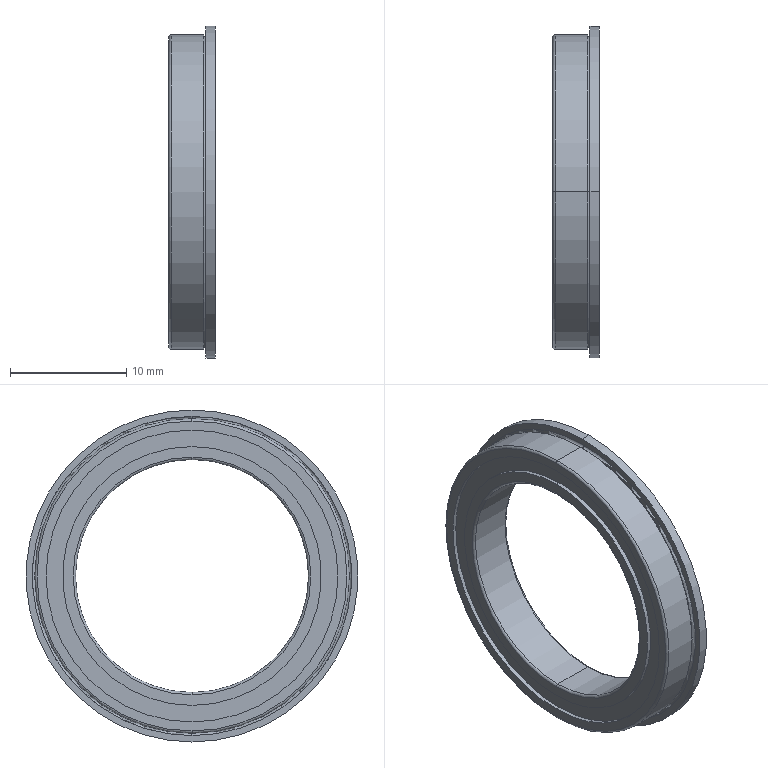Part | NX | features BREP 1 | 1 solid | 31 faces | box 4 x 28.5 x 28.5 mm | volume 1002 mm3 | cylinder 14 | torus 10 | plane 7 | commonest cylinder face diameters 22.21 x4 25.05 x4 20 x2 27 x2 28.5 x2
STEP:
#1=CARTESIAN_POINT('',(0.,0.,13.3));
#2=VERTEX_POINT('',#1);
#3=CARTESIAN_POINT('',(-0.2,0.,13.5));
#4=VERTEX_POINT('',#3);
#5=CARTESIAN_POINT('',(0.,0.,13.5));
#6=DIRECTION('',(0.,-1.,0.));
#7=DIRECTION('',(0.,0.,-1.));
#8=AXIS2_PLACEMENT_3D('',#5,#6,#7);
#9=CIRCLE('',#8,0.2);
#10=EDGE_CURVE('',#2,#4,#9,.F.);
#11=ORIENTED_EDGE('',*,*,#10,.F.);
#12=CARTESIAN_POINT('',(0.,0.,-13.3));
#13=VERTEX_POINT('',#12);
#14=CARTESIAN_POINT('',(0.,0.,0.));
#15=DIRECTION('',(-1.,0.,0.));
#16=DIRECTION('',(0.,0.,1.));
#17=AXIS2_PLACEMENT_3D('',#14,#15,#16);
#18=CIRCLE('',#17,13.3);
#19=EDGE_CURVE('',#2,#13,#18,.T.);
#20=ORIENTED_EDGE('',*,*,#19,.T.);
#21=CARTESIAN_POINT('',(-0.2,0.,-13.5));
#22=VERTEX_POINT('',#21);
#23=CARTESIAN_POINT('',(0.,0.,-13.5));
#24=DIRECTION('',(0.,1.,0.));
#25=DIRECTION('',(0.,0.,1.));
#26=AXIS2_PLACEMENT_3D('',#23,#24,#25);
#27=CIRCLE('',#26,0.2);
#28=EDGE_CURVE('',#13,#22,#27,.F.);
#29=ORIENTED_EDGE('',*,*,#28,.T.);
#30=CARTESIAN_POINT('',(-0.2,0.,0.));
#31=DIRECTION('',(-1.,0.,0.));
#32=DIRECTION('',(0.,0.,1.));
#33=AXIS2_PLACEMENT_3D('',#30,#31,#32);
#34=CIRCLE('',#33,13.5);
#35=EDGE_CURVE('',#4,#22,#34,.T.);
#36=ORIENTED_EDGE('',*,*,#35,.F.);
#37=EDGE_LOOP('',(#11,#20,#29,#36));
#38=FACE_BOUND('',#37,.T.);
#39=CARTESIAN_POINT('',(0.,0.,0.));
#40=DIRECTION('',(-1.,0.,0.));
#41=DIRECTION('',(0.,0.,-1.));
#42=AXIS2_PLACEMENT_3D('',#39,#40,#41);
#43=TOROIDAL_SURFACE('',#42,13.5,0.2);
#44=ADVANCED_FACE('',(#38),#43,.F.);
#45=ORIENTED_EDGE('',*,*,#28,.F.);
#46=CARTESIAN_POINT('',(0.,0.,0.));
#47=DIRECTION('',(-1.,0.,0.));
#48=DIRECTION('',(0.,0.,1.));
#49=AXIS2_PLACEMENT_3D('',#46,#47,#48);
#50=CIRCLE('',#49,13.3);
#51=EDGE_CURVE('',#13,#2,#50,.T.);
#52=ORIENTED_EDGE('',*,*,#51,.T.);
#53=ORIENTED_EDGE('',*,*,#10,.T.);
#54=CARTESIAN_POINT('',(-0.2,0.,0.));
#55=DIRECTION('',(-1.,0.,0.));
#56=DIRECTION('',(0.,0.,1.));
#57=AXIS2_PLACEMENT_3D('',#54,#55,#56);
#58=CIRCLE('',#57,13.5);
#59=EDGE_CURVE('',#22,#4,#58,.T.);
#60=ORIENTED_EDGE('',*,*,#59,.F.);
#61=EDGE_LOOP('',(#45,#52,#53,#60));
#62=FACE_BOUND('',#61,.T.);
#63=CARTESIAN_POINT('',(0.,0.,0.));
#64=DIRECTION('',(-1.,0.,0.));
#65=DIRECTION('',(0.,0.,-1.));
#66=AXIS2_PLACEMENT_3D('',#63,#64,#65);
#67=TOROIDAL_SURFACE('',#66,13.5,0.2);
#68=ADVANCED_FACE('',(#62),#67,.F.);
#69=CARTESIAN_POINT('',(-3.2,0.,13.3));
#70=VERTEX_POINT('',#69);
#71=CARTESIAN_POINT('',(-3.2,0.,-13.3));
#72=VERTEX_POINT('',#71);
#73=CARTESIAN_POINT('',(-3.2,0.,0.));
#74=DIRECTION('',(-1.,0.,0.));
#75=DIRECTION('',(0.,0.,-1.));
#76=AXIS2_PLACEMENT_3D('',#73,#74,#75);
#77=CIRCLE('',#76,13.3);
#78=EDGE_CURVE('',#70,#72,#77,.T.);
#79=ORIENTED_EDGE('',*,*,#78,.F.);
#80=CARTESIAN_POINT('',(-3.,0.,13.5));
#81=VERTEX_POINT('',#80);
#82=CARTESIAN_POINT('',(-3.,0.,13.3));
#83=DIRECTION('',(0.,1.,0.));
#84=DIRECTION('',(0.,0.,1.));
#85=AXIS2_PLACEMENT_3D('',#82,#83,#84);
#86=CIRCLE('',#85,0.2);
#87=EDGE_CURVE('',#81,#70,#86,.F.);
#88=ORIENTED_EDGE('',*,*,#87,.F.);
#89=CARTESIAN_POINT('',(-3.,0.,-13.5));
#90=VERTEX_POINT('',#89);
#91=CARTESIAN_POINT('',(-3.,0.,0.));
#92=DIRECTION('',(1.,0.,0.));
#93=DIRECTION('',(0.,0.,-1.));
#94=AXIS2_PLACEMENT_3D('',#91,#92,#93);
#95=CIRCLE('',#94,13.5);
#96=EDGE_CURVE('',#90,#81,#95,.T.);
#97=ORIENTED_EDGE('',*,*,#96,.F.);
#98=CARTESIAN_POINT('',(-3.,0.,-13.3));
#99=DIRECTION('',(0.,-1.,0.));
#100=DIRECTION('',(0.,0.,-1.));
#101=AXIS2_PLACEMENT_3D('',#98,#99,#100);
#102=CIRCLE('',#101,0.2);
#103=EDGE_CURVE('',#90,#72,#102,.F.);
#104=ORIENTED_EDGE('',*,*,#103,.T.);
#105=EDGE_LOOP('',(#79,#88,#97,#104));
#106=FACE_BOUND('',#105,.T.);
#107=CARTESIAN_POINT('',(-3.,0.,0.));
#108=DIRECTION('',(1.,0.,0.));
#109=DIRECTION('',(0.,0.,1.));
#110=AXIS2_PLACEMENT_3D('',#107,#108,#109);
#111=TOROIDAL_SURFACE('',#110,13.3,0.2);
#112=ADVANCED_FACE('',(#106),#111,.T.);
#113=CARTESIAN_POINT('',(-3.,0.,10.));
#114=VERTEX_POINT('',#113);
#115=CARTESIAN_POINT('',(-3.,0.,-10.));
#116=VERTEX_POINT('',#115);
#117=CARTESIAN_POINT('',(-3.,0.,0.));
#118=DIRECTION('',(-1.,0.,0.));
#119=DIRECTION('',(0.,0.,-1.));
#120=AXIS2_PLACEMENT_3D('',#117,#118,#119);
#121=CIRCLE('',#120,10.);
#122=EDGE_CURVE('',#114,#116,#121,.T.);
#123=ORIENTED_EDGE('',*,*,#122,.F.);
#124=CARTESIAN_POINT('',(-3.2,0.,10.2));
#125=VERTEX_POINT('',#124);
#126=CARTESIAN_POINT('',(-3.,0.,10.2));
#127=DIRECTION('',(0.,1.,0.));
#128=DIRECTION('',(0.,0.,1.));
#129=AXIS2_PLACEMENT_3D('',#126,#127,#128);
#130=CIRCLE('',#129,0.2);
#131=EDGE_CURVE('',#125,#114,#130,.F.);
#132=ORIENTED_EDGE('',*,*,#131,.F.);
#133=CARTESIAN_POINT('',(-3.2,0.,-10.2));
#134=VERTEX_POINT('',#133);
#135=CARTESIAN_POINT('',(-3.2,0.,0.));
#136=DIRECTION('',(1.,0.,0.));
#137=DIRECTION('',(0.,0.,-1.));
#138=AXIS2_PLACEMENT_3D('',#135,#136,#137);
#139=CIRCLE('',#138,10.2);
#140=EDGE_CURVE('',#134,#125,#139,.T.);
#141=ORIENTED_EDGE('',*,*,#140,.F.);
#142=CARTESIAN_POINT('',(-3.,0.,-10.2));
#143=DIRECTION('',(0.,-1.,0.));
#144=DIRECTION('',(0.,0.,-1.));
#145=AXIS2_PLACEMENT_3D('',#142,#143,#144);
#146=CIRCLE('',#145,0.2);
#147=EDGE_CURVE('',#134,#116,#146,.F.);
#148=ORIENTED_EDGE('',*,*,#147,.T.);
#149=EDGE_LOOP('',(#123,#132,#141,#148));
#150=FACE_BOUND('',#149,.T.);
#151=CARTESIAN_POINT('',(-3.,0.,0.));
#152=DIRECTION('',(1.,0.,0.));
#153=DIRECTION('',(0.,0.,1.));
#154=AXIS2_PLACEMENT_3D('',#151,#152,#153);
#155=TOROIDAL_SURFACE('',#154,10.2,0.2);
#156=ADVANCED_FACE('',(#150),#155,.T.);
#157=CARTESIAN_POINT('',(0.6,0.,-10.));
#158=VERTEX_POINT('',#157);
#159=CARTESIAN_POINT('',(0.6,0.,10.));
#160=VERTEX_POINT('',#159);
#161=CARTESIAN_POINT('',(0.6,0.,0.));
#162=DIRECTION('',(1.,0.,0.));
#163=DIRECTION('',(0.,0.,1.));
#164=AXIS2_PLACEMENT_3D('',#161,#162,#163);
#165=CIRCLE('',#164,10.);
#166=EDGE_CURVE('',#158,#160,#165,.T.);
#167=ORIENTED_EDGE('',*,*,#166,.F.);
#168=CARTESIAN_POINT('',(0.8,0.,-10.2));
#169=VERTEX_POINT('',#168);
#170=CARTESIAN_POINT('',(0.6,0.,-10.2));
#171=DIRECTION('',(0.,1.,0.));
#172=DIRECTION('',(0.,0.,1.));
#173=AXIS2_PLACEMENT_3D('',#170,#171,#172);
#174=CIRCLE('',#173,0.2);
#175=EDGE_CURVE('',#158,#169,#174,.T.);
#176=ORIENTED_EDGE('',*,*,#175,.T.);
#177=CARTESIAN_POINT('',(0.8,0.,10.2));
#178=VERTEX_POINT('',#177);
#179=CARTESIAN_POINT('',(0.8,0.,0.));
#180=DIRECTION('',(-1.,0.,0.));
#181=DIRECTION('',(0.,0.,1.));
#182=AXIS2_PLACEMENT_3D('',#179,#180,#181);
#183=CIRCLE('',#182,10.2);
#184=EDGE_CURVE('',#178,#169,#183,.T.);
#185=ORIENTED_EDGE('',*,*,#184,.F.);
#186=CARTESIAN_POINT('',(0.6,0.,10.2));
#187=DIRECTION('',(0.,-1.,0.));
#188=DIRECTION('',(0.,0.,-1.));
#189=AXIS2_PLACEMENT_3D('',#186,#187,#188);
#190=CIRCLE('',#189,0.2);
#191=EDGE_CURVE('',#160,#178,#190,.T.);
#192=ORIENTED_EDGE('',*,*,#191,.F.);
#193=EDGE_LOOP('',(#167,#176,#185,#192));
#194=FACE_BOUND('',#193,.T.);
#195=CARTESIAN_POINT('',(0.6,0.,0.));
#196=DIRECTION('',(-1.,0.,0.));
#197=DIRECTION('',(0.,0.,-1.));
#198=AXIS2_PLACEMENT_3D('',#195,#196,#197);
#199=TOROIDAL_SURFACE('',#198,10.2,0.2);
#200=ADVANCED_FACE('',(#194),#199,.T.);
#201=CARTESIAN_POINT('',(0.8,0.,-12.525));
#202=VERTEX_POINT('',#201);
#203=CARTESIAN_POINT('',(0.8,0.,12.525));
#204=VERTEX_POINT('',#203);
#205=CARTESIAN_POINT('',(0.8,0.,0.));
#206=DIRECTION('',(-1.,0.,0.));
#207=DIRECTION('',(0.,0.,1.));
#208=AXIS2_PLACEMENT_3D('',#205,#206,#207);
#209=CIRCLE('',#208,12.525);
#210=EDGE_CURVE('',#202,#204,#209,.T.);
#211=ORIENTED_EDGE('',*,*,#210,.F.);
#212=CARTESIAN_POINT('',(0.45,0.,-12.525));
#213=VERTEX_POINT('',#212);
#214=CARTESIAN_POINT('',(-3.2,0.,-12.525));
#215=DIRECTION('',(-1.,0.,0.));
#216=VECTOR('',#215,1000.);
#217=LINE('',#214,#216);
#218=EDGE_CURVE('',#202,#213,#217,.T.);
#219=ORIENTED_EDGE('',*,*,#218,.T.);
#220=CARTESIAN_POINT('',(0.45,0.,12.525));
#221=VERTEX_POINT('',#220);
#222=CARTESIAN_POINT('',(0.45,0.,0.));
#223=DIRECTION('',(-1.,0.,0.));
#224=DIRECTION('',(0.,0.,1.));
#225=AXIS2_PLACEMENT_3D('',#222,#223,#224);
#226=CIRCLE('',#225,12.525);
#227=EDGE_CURVE('',#213,#221,#226,.T.);
#228=ORIENTED_EDGE('',*,*,#227,.T.);
#229=CARTESIAN_POINT('',(-3.2,0.,12.525));
#230=DIRECTION('',(-1.,0.,0.));
#231=VECTOR('',#230,1000.);
#232=LINE('',#229,#231);
#233=EDGE_CURVE('',#204,#221,#232,.T.);
#234=ORIENTED_EDGE('',*,*,#233,.F.);
#235=EDGE_LOOP('',(#211,#219,#228,#234));
#236=FACE_BOUND('',#235,.T.);
#237=CARTESIAN_POINT('',(-3.2,0.,0.));
#238=DIRECTION('',(-1.,0.,0.));
#239=DIRECTION('',(0.,0.,-1.));
#240=AXIS2_PLACEMENT_3D('',#237,#238,#239);
#241=CYLINDRICAL_SURFACE('',#240,12.525);
#242=ADVANCED_FACE('',(#236),#241,.F.);
#243=CARTESIAN_POINT('',(0.8,0.,11.105));
#244=VERTEX_POINT('',#243);
#245=CARTESIAN_POINT('',(0.8,0.,-11.105));
#246=VERTEX_POINT('',#245);
#247=CARTESIAN_POINT('',(0.8,0.,0.));
#248=DIRECTION('',(-1.,0.,0.));
#249=DIRECTION('',(0.,0.,1.));
#250=AXIS2_PLACEMENT_3D('',#247,#248,#249);
#251=CIRCLE('',#250,11.105);
#252=EDGE_CURVE('',#244,#246,#251,.T.);
#253=ORIENTED_EDGE('',*,*,#252,.T.);
#254=CARTESIAN_POINT('',(0.45,0.,-11.105));
#255=VERTEX_POINT('',#254);
#256=CARTESIAN_POINT('',(-3.2,0.,-11.105));
#257=DIRECTION('',(-1.,0.,0.));
#258=VECTOR('',#257,1000.);
#259=LINE('',#256,#258);
#260=EDGE_CURVE('',#246,#255,#259,.T.);
#261=ORIENTED_EDGE('',*,*,#260,.T.);
#262=CARTESIAN_POINT('',(0.45,0.,11.105));
#263=VERTEX_POINT('',#262);
#264=CARTESIAN_POINT('',(0.45,0.,0.));
#265=DIRECTION('',(-1.,0.,0.));
#266=DIRECTION('',(0.,0.,1.));
#267=AXIS2_PLACEMENT_3D('',#264,#265,#266);
#268=CIRCLE('',#267,11.105);
#269=EDGE_CURVE('',#263,#255,#268,.T.);
#270=ORIENTED_EDGE('',*,*,#269,.F.);
#271=CARTESIAN_POINT('',(-3.2,0.,11.105));
#272=DIRECTION('',(-1.,0.,0.));
#273=VECTOR('',#272,1000.);
#274=LINE('',#271,#273);
#275=EDGE_CURVE('',#244,#263,#274,.T.);
#276=ORIENTED_EDGE('',*,*,#275,.F.);
#277=EDGE_LOOP('',(#253,#261,#270,#276));
#278=FACE_BOUND('',#277,.T.);
#279=CARTESIAN_POINT('',(-3.2,0.,0.));
#280=DIRECTION('',(-1.,0.,0.));
#281=DIRECTION('',(0.,0.,-1.));
#282=AXIS2_PLACEMENT_3D('',#279,#280,#281);
#283=CYLINDRICAL_SURFACE('',#282,11.105);
#284=ADVANCED_FACE('',(#278),#283,.T.);
#285=CARTESIAN_POINT('',(0.6,0.,0.));
#286=DIRECTION('',(1.,0.,0.));
#287=DIRECTION('',(0.,0.,1.));
#288=AXIS2_PLACEMENT_3D('',#285,#286,#287);
#289=CIRCLE('',#288,10.);
#290=EDGE_CURVE('',#160,#158,#289,.T.);
#291=ORIENTED_EDGE('',*,*,#290,.T.);
#292=CARTESIAN_POINT('',(-3.2,0.,-10.));
#293=DIRECTION('',(-1.,0.,0.));
#294=VECTOR('',#293,1000.);
#295=LINE('',#292,#294);
#296=EDGE_CURVE('',#158,#116,#295,.T.);
#297=ORIENTED_EDGE('',*,*,#296,.T.);
#298=CARTESIAN_POINT('',(-3.,0.,0.));
#299=DIRECTION('',(-1.,0.,0.));
#300=DIRECTION('',(0.,0.,-1.));
#301=AXIS2_PLACEMENT_3D('',#298,#299,#300);
#302=CIRCLE('',#301,10.);
#303=EDGE_CURVE('',#116,#114,#302,.T.);
#304=ORIENTED_EDGE('',*,*,#303,.T.);
#305=CARTESIAN_POINT('',(-3.2,0.,10.));
#306=DIRECTION('',(-1.,0.,0.));
#307=VECTOR('',#306,1000.);
#308=LINE('',#305,#307);
#309=EDGE_CURVE('',#160,#114,#308,.T.);
#310=ORIENTED_EDGE('',*,*,#309,.F.);
#311=EDGE_LOOP('',(#291,#297,#304,#310));
#312=FACE_BOUND('',#311,.T.);
#313=CARTESIAN_POINT('',(-3.2,0.,0.));
#314=DIRECTION('',(-1.,0.,0.));
#315=DIRECTION('',(0.,0.,-1.));
#316=AXIS2_PLACEMENT_3D('',#313,#314,#315);
#317=CYLINDRICAL_SURFACE('',#316,10.);
#318=ADVANCED_FACE('',(#312),#317,.F.);
#319=CARTESIAN_POINT('',(-2.85,0.,11.105));
#320=VERTEX_POINT('',#319);
#321=CARTESIAN_POINT('',(-2.85,0.,-11.105));
#322=VERTEX_POINT('',#321);
#323=CARTESIAN_POINT('',(-2.85,0.,0.));
#324=DIRECTION('',(-1.,0.,0.));
#325=DIRECTION('',(0.,0.,1.));
#326=AXIS2_PLACEMENT_3D('',#323,#324,#325);
#327=CIRCLE('',#326,11.105);
#328=EDGE_CURVE('',#320,#322,#327,.T.);
#329=ORIENTED_EDGE('',*,*,#328,.T.);
#330=CARTESIAN_POINT('',(-3.2,0.,-11.105));
#331=VERTEX_POINT('',#330);
#332=CARTESIAN_POINT('',(-3.2,0.,-11.105));
#333=DIRECTION('',(-1.,0.,0.));
#334=VECTOR('',#333,1000.);
#335=LINE('',#332,#334);
#336=EDGE_CURVE('',#322,#331,#335,.T.);
#337=ORIENTED_EDGE('',*,*,#336,.T.);
#338=CARTESIAN_POINT('',(-3.2,0.,11.105));
#339=VERTEX_POINT('',#338);
#340=CARTESIAN_POINT('',(-3.2,0.,0.));
#341=DIRECTION('',(-1.,0.,0.));
#342=DIRECTION('',(0.,0.,1.));
#343=AXIS2_PLACEMENT_3D('',#340,#341,#342);
#344=CIRCLE('',#343,11.105);
#345=EDGE_CURVE('',#339,#331,#344,.T.);
#346=ORIENTED_EDGE('',*,*,#345,.F.);
#347=CARTESIAN_POINT('',(-3.2,0.,11.105));
#348=DIRECTION('',(-1.,0.,0.));
#349=VECTOR('',#348,1000.);
#350=LINE('',#347,#349);
#351=EDGE_CURVE('',#320,#339,#350,.T.);
#352=ORIENTED_EDGE('',*,*,#351,.F.);
#353=EDGE_LOOP('',(#329,#337,#346,#352));
#354=FACE_BOUND('',#353,.T.);
#355=CARTESIAN_POINT('',(-3.2,0.,0.));
#356=DIRECTION('',(-1.,0.,0.));
#357=DIRECTION('',(0.,0.,-1.));
#358=AXIS2_PLACEMENT_3D('',#355,#356,#357);
#359=CYLINDRICAL_SURFACE('',#358,11.105);
#360=ADVANCED_FACE('',(#354),#359,.T.);
#361=CARTESIAN_POINT('',(-2.85,0.,-12.525));
#362=VERTEX_POINT('',#361);
#363=CARTESIAN_POINT('',(-2.85,0.,12.525));
#364=VERTEX_POINT('',#363);
#365=CARTESIAN_POINT('',(-2.85,0.,0.));
#366=DIRECTION('',(-1.,0.,0.));
#367=DIRECTION('',(0.,0.,1.));
#368=AXIS2_PLACEMENT_3D('',#365,#366,#367);
#369=CIRCLE('',#368,12.525);
#370=EDGE_CURVE('',#362,#364,#369,.T.);
#371=ORIENTED_EDGE('',*,*,#370,.F.);
#372=CARTESIAN_POINT('',(-3.2,0.,-12.525));
#373=VERTEX_POINT('',#372);
#374=CARTESIAN_POINT('',(-3.2,0.,-12.525));
#375=DIRECTION('',(-1.,0.,0.));
#376=VECTOR('',#375,1000.);
#377=LINE('',#374,#376);
#378=EDGE_CURVE('',#362,#373,#377,.T.);
#379=ORIENTED_EDGE('',*,*,#378,.T.);
#380=CARTESIAN_POINT('',(-3.2,0.,12.525));
#381=VERTEX_POINT('',#380);
#382=CARTESIAN_POINT('',(-3.2,0.,0.));
#383=DIRECTION('',(-1.,0.,0.));
#384=DIRECTION('',(0.,0.,1.));
#385=AXIS2_PLACEMENT_3D('',#382,#383,#384);
#386=CIRCLE('',#385,12.525);
#387=EDGE_CURVE('',#373,#381,#386,.T.);
#388=ORIENTED_EDGE('',*,*,#387,.T.);
#389=CARTESIAN_POINT('',(-3.2,0.,12.525));
#390=DIRECTION('',(-1.,0.,0.));
#391=VECTOR('',#390,1000.);
#392=LINE('',#389,#391);
#393=EDGE_CURVE('',#364,#381,#392,.T.);
#394=ORIENTED_EDGE('',*,*,#393,.F.);
#395=EDGE_LOOP('',(#371,#379,#388,#394));
#396=FACE_BOUND('',#395,.T.);
#397=CARTESIAN_POINT('',(-3.2,0.,0.));
#398=DIRECTION('',(-1.,0.,0.));
#399=DIRECTION('',(0.,0.,-1.));
#400=AXIS2_PLACEMENT_3D('',#397,#398,#399);
#401=CYLINDRICAL_SURFACE('',#400,12.525);
#402=ADVANCED_FACE('',(#396),#401,.F.);
#403=ORIENTED_EDGE('',*,*,#35,.T.);
#404=CARTESIAN_POINT('',(-3.2,0.,-13.5));
#405=DIRECTION('',(-1.,0.,0.));
#406=VECTOR('',#405,1000.);
#407=LINE('',#404,#406);
#408=EDGE_CURVE('',#22,#90,#407,.T.);
#409=ORIENTED_EDGE('',*,*,#408,.T.);
#410=ORIENTED_EDGE('',*,*,#96,.T.);
#411=CARTESIAN_POINT('',(-3.2,0.,13.5));
#412=DIRECTION('',(-1.,0.,0.));
#413=VECTOR('',#412,1000.);
#414=LINE('',#411,#413);
#415=EDGE_CURVE('',#4,#81,#414,.T.);
#416=ORIENTED_EDGE('',*,*,#415,.F.);
#417=EDGE_LOOP('',(#403,#409,#410,#416));
#418=FACE_BOUND('',#417,.T.);
#419=CARTESIAN_POINT('',(-3.2,0.,0.));
#420=DIRECTION('',(-1.,0.,0.));
#421=DIRECTION('',(0.,0.,-1.));
#422=AXIS2_PLACEMENT_3D('',#419,#420,#421);
#423=CYLINDRICAL_SURFACE('',#422,13.5);
#424=ADVANCED_FACE('',(#418),#423,.T.);
#425=ORIENTED_EDGE('',*,*,#51,.F.);
#426=CARTESIAN_POINT('',(0.,0.,-13.7));
#427=VERTEX_POINT('',#426);
#428=CARTESIAN_POINT('',(0.,0.,-13.5));
#429=DIRECTION('',(0.,1.,0.));
#430=DIRECTION('',(0.,0.,1.));
#431=AXIS2_PLACEMENT_3D('',#428,#429,#430);
#432=CIRCLE('',#431,0.2);
#433=EDGE_CURVE('',#13,#427,#432,.T.);
#434=ORIENTED_EDGE('',*,*,#433,.T.);
#435=CARTESIAN_POINT('',(0.,0.,13.7));
#436=VERTEX_POINT('',#435);
#437=CARTESIAN_POINT('',(0.,0.,0.));
#438=DIRECTION('',(-1.,0.,0.));
#439=DIRECTION('',(0.,0.,1.));
#440=AXIS2_PLACEMENT_3D('',#437,#438,#439);
#441=CIRCLE('',#440,13.7);
#442=EDGE_CURVE('',#427,#436,#441,.T.);
#443=ORIENTED_EDGE('',*,*,#442,.T.);
#444=CARTESIAN_POINT('',(0.,0.,13.5));
#445=DIRECTION('',(0.,-1.,0.));
#446=DIRECTION('',(0.,0.,-1.));
#447=AXIS2_PLACEMENT_3D('',#444,#445,#446);
#448=CIRCLE('',#447,0.2);
#449=EDGE_CURVE('',#2,#436,#448,.T.);
#450=ORIENTED_EDGE('',*,*,#449,.F.);
#451=EDGE_LOOP('',(#425,#434,#443,#450));
#452=FACE_BOUND('',#451,.T.);
#453=CARTESIAN_POINT('',(0.,0.,0.));
#454=DIRECTION('',(-1.,0.,0.));
#455=DIRECTION('',(0.,0.,-1.));
#456=AXIS2_PLACEMENT_3D('',#453,#454,#455);
#457=TOROIDAL_SURFACE('',#456,13.5,0.2);
#458=ADVANCED_FACE('',(#452),#457,.F.);
#459=CARTESIAN_POINT('',(0.8,0.,14.25));
#460=VERTEX_POINT('',#459);
#461=CARTESIAN_POINT('',(0.8,0.,-14.25));
#462=VERTEX_POINT('',#461);
#463=CARTESIAN_POINT('',(0.8,0.,0.));
#464=DIRECTION('',(-1.,0.,0.));
#465=DIRECTION('',(0.,0.,1.));
#466=AXIS2_PLACEMENT_3D('',#463,#464,#465);
#467=CIRCLE('',#466,14.25);
#468=EDGE_CURVE('',#460,#462,#467,.T.);
#469=ORIENTED_EDGE('',*,*,#468,.T.);
#470=CARTESIAN_POINT('',(0.,0.,-14.25));
#471=VERTEX_POINT('',#470);
#472=CARTESIAN_POINT('',(-3.2,0.,-14.25));
#473=DIRECTION('',(-1.,0.,0.));
#474=VECTOR('',#473,1000.);
#475=LINE('',#472,#474);
#476=EDGE_CURVE('',#462,#471,#475,.T.);
#477=ORIENTED_EDGE('',*,*,#476,.T.);
#478=CARTESIAN_POINT('',(0.,0.,14.25));
#479=VERTEX_POINT('',#478);
#480=CARTESIAN_POINT('',(0.,0.,0.));
#481=DIRECTION('',(-1.,0.,0.));
#482=DIRECTION('',(0.,0.,1.));
#483=AXIS2_PLACEMENT_3D('',#480,#481,#482);
#484=CIRCLE('',#483,14.25);
#485=EDGE_CURVE('',#479,#471,#484,.T.);
#486=ORIENTED_EDGE('',*,*,#485,.F.);
#487=CARTESIAN_POINT('',(-3.2,0.,14.25));
#488=DIRECTION('',(-1.,0.,0.));
#489=VECTOR('',#488,1000.);
#490=LINE('',#487,#489);
#491=EDGE_CURVE('',#460,#479,#490,.T.);
#492=ORIENTED_EDGE('',*,*,#491,.F.);
#493=EDGE_LOOP('',(#469,#477,#486,#492));
#494=FACE_BOUND('',#493,.T.);
#495=CARTESIAN_POINT('',(-3.2,0.,0.));
#496=DIRECTION('',(-1.,0.,0.));
#497=DIRECTION('',(0.,0.,-1.));
#498=AXIS2_PLACEMENT_3D('',#495,#496,#497);
#499=CYLINDRICAL_SURFACE('',#498,14.25);
#500=ADVANCED_FACE('',(#494),#499,.T.);
#501=ORIENTED_EDGE('',*,*,#476,.F.);
#502=CARTESIAN_POINT('',(0.8,0.,0.));
#503=DIRECTION('',(-1.,0.,0.));
#504=DIRECTION('',(0.,0.,1.));
#505=AXIS2_PLACEMENT_3D('',#502,#503,#504);
#506=CIRCLE('',#505,14.25);
#507=EDGE_CURVE('',#462,#460,#506,.T.);
#508=ORIENTED_EDGE('',*,*,#507,.T.);
#509=ORIENTED_EDGE('',*,*,#491,.T.);
#510=CARTESIAN_POINT('',(0.,0.,0.));
#511=DIRECTION('',(-1.,0.,0.));
#512=DIRECTION('',(0.,0.,1.));
#513=AXIS2_PLACEMENT_3D('',#510,#511,#512);
#514=CIRCLE('',#513,14.25);
#515=EDGE_CURVE('',#471,#479,#514,.T.);
#516=ORIENTED_EDGE('',*,*,#515,.F.);
#517=EDGE_LOOP('',(#501,#508,#509,#516));
#518=FACE_BOUND('',#517,.T.);
#519=CARTESIAN_POINT('',(-3.2,0.,0.));
#520=DIRECTION('',(-1.,0.,0.));
#521=DIRECTION('',(0.,0.,-1.));
#522=AXIS2_PLACEMENT_3D('',#519,#520,#521);
#523=CYLINDRICAL_SURFACE('',#522,14.25);
#524=ADVANCED_FACE('',(#518),#523,.T.);
#525=ORIENTED_EDGE('',*,*,#485,.T.);
#526=ORIENTED_EDGE('',*,*,#515,.T.);
#527=EDGE_LOOP('',(#525,#526));
#528=FACE_BOUND('',#527,.T.);
#529=CARTESIAN_POINT('',(0.,0.,0.));
#530=DIRECTION('',(-1.,0.,0.));
#531=DIRECTION('',(0.,0.,1.));
#532=AXIS2_PLACEMENT_3D('',#529,#530,#531);
#533=CIRCLE('',#532,13.7);
#534=EDGE_CURVE('',#436,#427,#533,.T.);
#535=ORIENTED_EDGE('',*,*,#534,.F.);
#536=ORIENTED_EDGE('',*,*,#442,.F.);
#537=EDGE_LOOP('',(#535,#536));
#538=FACE_BOUND('',#537,.T.);
#539=CARTESIAN_POINT('',(0.,13.7,0.));
#540=DIRECTION('',(1.,0.,0.));
#541=DIRECTION('',(0.,-1.,0.));
#542=AXIS2_PLACEMENT_3D('',#539,#540,#541);
#543=PLANE('',#542);
#544=ADVANCED_FACE('',(#528,#538),#543,.F.);
#545=ORIENTED_EDGE('',*,*,#19,.F.);
#546=ORIENTED_EDGE('',*,*,#449,.T.);
#547=ORIENTED_EDGE('',*,*,#534,.T.);
#548=ORIENTED_EDGE('',*,*,#433,.F.);
#549=EDGE_LOOP('',(#545,#546,#547,#548));
#550=FACE_BOUND('',#549,.T.);
#551=CARTESIAN_POINT('',(0.,0.,0.));
#552=DIRECTION('',(-1.,0.,0.));
#553=DIRECTION('',(0.,0.,-1.));
#554=AXIS2_PLACEMENT_3D('',#551,#552,#553);
#555=TOROIDAL_SURFACE('',#554,13.5,0.2);
#556=ADVANCED_FACE('',(#550),#555,.F.);
#557=ORIENTED_EDGE('',*,*,#408,.F.);
#558=ORIENTED_EDGE('',*,*,#59,.T.);
#559=ORIENTED_EDGE('',*,*,#415,.T.);
#560=CARTESIAN_POINT('',(-3.,0.,0.));
#561=DIRECTION('',(1.,0.,0.));
#562=DIRECTION('',(0.,0.,-1.));
#563=AXIS2_PLACEMENT_3D('',#560,#561,#562);
#564=CIRCLE('',#563,13.5);
#565=EDGE_CURVE('',#81,#90,#564,.T.);
#566=ORIENTED_EDGE('',*,*,#565,.T.);
#567=EDGE_LOOP('',(#557,#558,#559,#566));
#568=FACE_BOUND('',#567,.T.);
#569=CARTESIAN_POINT('',(-3.2,0.,0.));
#570=DIRECTION('',(-1.,0.,0.));
#571=DIRECTION('',(0.,0.,-1.));
#572=AXIS2_PLACEMENT_3D('',#569,#570,#571);
#573=CYLINDRICAL_SURFACE('',#572,13.5);
#574=ADVANCED_FACE('',(#568),#573,.T.);
#575=CARTESIAN_POINT('',(-3.2,0.,0.));
#576=DIRECTION('',(-1.,0.,0.));
#577=DIRECTION('',(0.,0.,-1.));
#578=AXIS2_PLACEMENT_3D('',#575,#576,#577);
#579=CIRCLE('',#578,13.3);
#580=EDGE_CURVE('',#72,#70,#579,.T.);
#581=ORIENTED_EDGE('',*,*,#580,.T.);
#582=ORIENTED_EDGE('',*,*,#78,.T.);
#583=EDGE_LOOP('',(#581,#582));
#584=FACE_BOUND('',#583,.T.);
#585=CARTESIAN_POINT('',(-3.2,0.,0.));
#586=DIRECTION('',(-1.,0.,0.));
#587=DIRECTION('',(0.,0.,1.));
#588=AXIS2_PLACEMENT_3D('',#585,#586,#587);
#589=CIRCLE('',#588,12.525);
#590=EDGE_CURVE('',#381,#373,#589,.T.);
#591=ORIENTED_EDGE('',*,*,#590,.F.);
#592=ORIENTED_EDGE('',*,*,#387,.F.);
#593=EDGE_LOOP('',(#591,#592));
#594=FACE_BOUND('',#593,.T.);
#595=CARTESIAN_POINT('',(-3.2,12.525,0.));
#596=DIRECTION('',(1.,0.,0.));
#597=DIRECTION('',(0.,-1.,0.));
#598=AXIS2_PLACEMENT_3D('',#595,#596,#597);
#599=PLANE('',#598);
#600=ADVANCED_FACE('',(#584,#594),#599,.F.);
#601=ORIENTED_EDGE('',*,*,#378,.F.);
#602=CARTESIAN_POINT('',(-2.85,0.,0.));
#603=DIRECTION('',(-1.,0.,0.));
#604=DIRECTION('',(0.,0.,1.));
#605=AXIS2_PLACEMENT_3D('',#602,#603,#604);
#606=CIRCLE('',#605,12.525);
#607=EDGE_CURVE('',#364,#362,#606,.T.);
#608=ORIENTED_EDGE('',*,*,#607,.F.);
#609=ORIENTED_EDGE('',*,*,#393,.T.);
#610=ORIENTED_EDGE('',*,*,#590,.T.);
#611=EDGE_LOOP('',(#601,#608,#609,#610));
#612=FACE_BOUND('',#611,.T.);
#613=CARTESIAN_POINT('',(-3.2,0.,0.));
#614=DIRECTION('',(-1.,0.,0.));
#615=DIRECTION('',(0.,0.,-1.));
#616=AXIS2_PLACEMENT_3D('',#613,#614,#615);
#617=CYLINDRICAL_SURFACE('',#616,12.525);
#618=ADVANCED_FACE('',(#612),#617,.F.);
#619=ORIENTED_EDGE('',*,*,#607,.T.);
#620=ORIENTED_EDGE('',*,*,#370,.T.);
#621=EDGE_LOOP('',(#619,#620));
#622=FACE_BOUND('',#621,.T.);
#623=ORIENTED_EDGE('',*,*,#328,.F.);
#624=CARTESIAN_POINT('',(-2.85,0.,0.));
#625=DIRECTION('',(-1.,0.,0.));
#626=DIRECTION('',(0.,0.,1.));
#627=AXIS2_PLACEMENT_3D('',#624,#625,#626);
#628=CIRCLE('',#627,11.105);
#629=EDGE_CURVE('',#322,#320,#628,.T.);
#630=ORIENTED_EDGE('',*,*,#629,.F.);
#631=EDGE_LOOP('',(#623,#630));
#632=FACE_BOUND('',#631,.T.);
#633=CARTESIAN_POINT('',(-2.85,12.525,0.));
#634=DIRECTION('',(1.,0.,0.));
#635=DIRECTION('',(0.,-1.,0.));
#636=AXIS2_PLACEMENT_3D('',#633,#634,#635);
#637=PLANE('',#636);
#638=ADVANCED_FACE('',(#622,#632),#637,.F.);
#639=ORIENTED_EDGE('',*,*,#336,.F.);
#640=ORIENTED_EDGE('',*,*,#629,.T.);
#641=ORIENTED_EDGE('',*,*,#351,.T.);
#642=CARTESIAN_POINT('',(-3.2,0.,0.));
#643=DIRECTION('',(-1.,0.,0.));
#644=DIRECTION('',(0.,0.,1.));
#645=AXIS2_PLACEMENT_3D('',#642,#643,#644);
#646=CIRCLE('',#645,11.105);
#647=EDGE_CURVE('',#331,#339,#646,.T.);
#648=ORIENTED_EDGE('',*,*,#647,.F.);
#649=EDGE_LOOP('',(#639,#640,#641,#648));
#650=FACE_BOUND('',#649,.T.);
#651=CARTESIAN_POINT('',(-3.2,0.,0.));
#652=DIRECTION('',(-1.,0.,0.));
#653=DIRECTION('',(0.,0.,-1.));
#654=AXIS2_PLACEMENT_3D('',#651,#652,#653);
#655=CYLINDRICAL_SURFACE('',#654,11.105);
#656=ADVANCED_FACE('',(#650),#655,.T.);
#657=ORIENTED_EDGE('',*,*,#345,.T.);
#658=ORIENTED_EDGE('',*,*,#647,.T.);
#659=EDGE_LOOP('',(#657,#658));
#660=FACE_BOUND('',#659,.T.);
#661=ORIENTED_EDGE('',*,*,#140,.T.);
#662=CARTESIAN_POINT('',(-3.2,0.,0.));
#663=DIRECTION('',(1.,0.,0.));
#664=DIRECTION('',(0.,0.,-1.));
#665=AXIS2_PLACEMENT_3D('',#662,#663,#664);
#666=CIRCLE('',#665,10.2);
#667=EDGE_CURVE('',#125,#134,#666,.T.);
#668=ORIENTED_EDGE('',*,*,#667,.T.);
#669=EDGE_LOOP('',(#661,#668));
#670=FACE_BOUND('',#669,.T.);
#671=CARTESIAN_POINT('',(-3.2,10.,0.));
#672=DIRECTION('',(1.,0.,0.));
#673=DIRECTION('',(0.,-1.,0.));
#674=AXIS2_PLACEMENT_3D('',#671,#672,#673);
#675=PLANE('',#674);
#676=ADVANCED_FACE('',(#660,#670),#675,.F.);
#677=ORIENTED_EDGE('',*,*,#296,.F.);
#678=ORIENTED_EDGE('',*,*,#166,.T.);
#679=ORIENTED_EDGE('',*,*,#309,.T.);
#680=ORIENTED_EDGE('',*,*,#122,.T.);
#681=EDGE_LOOP('',(#677,#678,#679,#680));
#682=FACE_BOUND('',#681,.T.);
#683=CARTESIAN_POINT('',(-3.2,0.,0.));
#684=DIRECTION('',(-1.,0.,0.));
#685=DIRECTION('',(0.,0.,-1.));
#686=AXIS2_PLACEMENT_3D('',#683,#684,#685);
#687=CYLINDRICAL_SURFACE('',#686,10.);
#688=ADVANCED_FACE('',(#682),#687,.F.);
#689=ORIENTED_EDGE('',*,*,#252,.F.);
#690=CARTESIAN_POINT('',(0.8,0.,0.));
#691=DIRECTION('',(-1.,0.,0.));
#692=DIRECTION('',(0.,0.,1.));
#693=AXIS2_PLACEMENT_3D('',#690,#691,#692);
#694=CIRCLE('',#693,11.105);
#695=EDGE_CURVE('',#246,#244,#694,.T.);
#696=ORIENTED_EDGE('',*,*,#695,.F.);
#697=EDGE_LOOP('',(#689,#696));
#698=FACE_BOUND('',#697,.T.);
#699=ORIENTED_EDGE('',*,*,#184,.T.);
#700=CARTESIAN_POINT('',(0.8,0.,0.));
#701=DIRECTION('',(-1.,0.,0.));
#702=DIRECTION('',(0.,0.,1.));
#703=AXIS2_PLACEMENT_3D('',#700,#701,#702);
#704=CIRCLE('',#703,10.2);
#705=EDGE_CURVE('',#169,#178,#704,.T.);
#706=ORIENTED_EDGE('',*,*,#705,.T.);
#707=EDGE_LOOP('',(#699,#706));
#708=FACE_BOUND('',#707,.T.);
#709=CARTESIAN_POINT('',(0.8,11.105,0.));
#710=DIRECTION('',(-1.,0.,0.));
#711=DIRECTION('',(0.,0.,-1.));
#712=AXIS2_PLACEMENT_3D('',#709,#710,#711);
#713=PLANE('',#712);
#714=ADVANCED_FACE('',(#698,#708),#713,.F.);
#715=ORIENTED_EDGE('',*,*,#260,.F.);
#716=ORIENTED_EDGE('',*,*,#695,.T.);
#717=ORIENTED_EDGE('',*,*,#275,.T.);
#718=CARTESIAN_POINT('',(0.45,0.,0.));
#719=DIRECTION('',(-1.,0.,0.));
#720=DIRECTION('',(0.,0.,1.));
#721=AXIS2_PLACEMENT_3D('',#718,#719,#720);
#722=CIRCLE('',#721,11.105);
#723=EDGE_CURVE('',#255,#263,#722,.T.);
#724=ORIENTED_EDGE('',*,*,#723,.F.);
#725=EDGE_LOOP('',(#715,#716,#717,#724));
#726=FACE_BOUND('',#725,.T.);
#727=CARTESIAN_POINT('',(-3.2,0.,0.));
#728=DIRECTION('',(-1.,0.,0.));
#729=DIRECTION('',(0.,0.,-1.));
#730=AXIS2_PLACEMENT_3D('',#727,#728,#729);
#731=CYLINDRICAL_SURFACE('',#730,11.105);
#732=ADVANCED_FACE('',(#726),#731,.T.);
#733=CARTESIAN_POINT('',(0.45,0.,0.));
#734=DIRECTION('',(-1.,0.,0.));
#735=DIRECTION('',(0.,0.,1.));
#736=AXIS2_PLACEMENT_3D('',#733,#734,#735);
#737=CIRCLE('',#736,12.525);
#738=EDGE_CURVE('',#221,#213,#737,.T.);
#739=ORIENTED_EDGE('',*,*,#738,.F.);
#740=ORIENTED_EDGE('',*,*,#227,.F.);
#741=EDGE_LOOP('',(#739,#740));
#742=FACE_BOUND('',#741,.T.);
#743=ORIENTED_EDGE('',*,*,#269,.T.);
#744=ORIENTED_EDGE('',*,*,#723,.T.);
#745=EDGE_LOOP('',(#743,#744));
#746=FACE_BOUND('',#745,.T.);
#747=CARTESIAN_POINT('',(0.45,12.525,0.));
#748=DIRECTION('',(-1.,0.,0.));
#749=DIRECTION('',(0.,0.,-1.));
#750=AXIS2_PLACEMENT_3D('',#747,#748,#749);
#751=PLANE('',#750);
#752=ADVANCED_FACE('',(#742,#746),#751,.F.);
#753=ORIENTED_EDGE('',*,*,#218,.F.);
#754=CARTESIAN_POINT('',(0.8,0.,0.));
#755=DIRECTION('',(-1.,0.,0.));
#756=DIRECTION('',(0.,0.,1.));
#757=AXIS2_PLACEMENT_3D('',#754,#755,#756);
#758=CIRCLE('',#757,12.525);
#759=EDGE_CURVE('',#204,#202,#758,.T.);
#760=ORIENTED_EDGE('',*,*,#759,.F.);
#761=ORIENTED_EDGE('',*,*,#233,.T.);
#762=ORIENTED_EDGE('',*,*,#738,.T.);
#763=EDGE_LOOP('',(#753,#760,#761,#762));
#764=FACE_BOUND('',#763,.T.);
#765=CARTESIAN_POINT('',(-3.2,0.,0.));
#766=DIRECTION('',(-1.,0.,0.));
#767=DIRECTION('',(0.,0.,-1.));
#768=AXIS2_PLACEMENT_3D('',#765,#766,#767);
#769=CYLINDRICAL_SURFACE('',#768,12.525);
#770=ADVANCED_FACE('',(#764),#769,.F.);
#771=ORIENTED_EDGE('',*,*,#468,.F.);
#772=ORIENTED_EDGE('',*,*,#507,.F.);
#773=EDGE_LOOP('',(#771,#772));
#774=FACE_BOUND('',#773,.T.);
#775=ORIENTED_EDGE('',*,*,#759,.T.);
#776=ORIENTED_EDGE('',*,*,#210,.T.);
#777=EDGE_LOOP('',(#775,#776));
#778=FACE_BOUND('',#777,.T.);
#779=CARTESIAN_POINT('',(0.8,14.25,0.));
#780=DIRECTION('',(-1.,0.,0.));
#781=DIRECTION('',(0.,0.,-1.));
#782=AXIS2_PLACEMENT_3D('',#779,#780,#781);
#783=PLANE('',#782);
#784=ADVANCED_FACE('',(#774,#778),#783,.F.);
#785=ORIENTED_EDGE('',*,*,#175,.F.);
#786=ORIENTED_EDGE('',*,*,#290,.F.);
#787=ORIENTED_EDGE('',*,*,#191,.T.);
#788=ORIENTED_EDGE('',*,*,#705,.F.);
#789=EDGE_LOOP('',(#785,#786,#787,#788));
#790=FACE_BOUND('',#789,.T.);
#791=CARTESIAN_POINT('',(0.6,0.,0.));
#792=DIRECTION('',(-1.,0.,0.));
#793=DIRECTION('',(0.,0.,-1.));
#794=AXIS2_PLACEMENT_3D('',#791,#792,#793);
#795=TOROIDAL_SURFACE('',#794,10.2,0.2);
#796=ADVANCED_FACE('',(#790),#795,.T.);
#797=ORIENTED_EDGE('',*,*,#131,.T.);
#798=ORIENTED_EDGE('',*,*,#303,.F.);
#799=ORIENTED_EDGE('',*,*,#147,.F.);
#800=ORIENTED_EDGE('',*,*,#667,.F.);
#801=EDGE_LOOP('',(#797,#798,#799,#800));
#802=FACE_BOUND('',#801,.T.);
#803=CARTESIAN_POINT('',(-3.,0.,0.));
#804=DIRECTION('',(1.,0.,0.));
#805=DIRECTION('',(0.,0.,1.));
#806=AXIS2_PLACEMENT_3D('',#803,#804,#805);
#807=TOROIDAL_SURFACE('',#806,10.2,0.2);
#808=ADVANCED_FACE('',(#802),#807,.T.);
#809=ORIENTED_EDGE('',*,*,#87,.T.);
#810=ORIENTED_EDGE('',*,*,#580,.F.);
#811=ORIENTED_EDGE('',*,*,#103,.F.);
#812=ORIENTED_EDGE('',*,*,#565,.F.);
#813=EDGE_LOOP('',(#809,#810,#811,#812));
#814=FACE_BOUND('',#813,.T.);
#815=CARTESIAN_POINT('',(-3.,0.,0.));
#816=DIRECTION('',(1.,0.,0.));
#817=DIRECTION('',(0.,0.,1.));
#818=AXIS2_PLACEMENT_3D('',#815,#816,#817);
#819=TOROIDAL_SURFACE('',#818,13.3,0.2);
#820=ADVANCED_FACE('',(#814),#819,.T.);
#821=CLOSED_SHELL('',(#44,#68,#112,#156,#200,#242,#284,#318,#360,#402,#424,#458,#500,#524,#544,#556,#574,#600,#618,#638,#656,#676,#688,#714,#732,#752,#770,#784,#796,#808,#820));
#822=MANIFOLD_SOLID_BREP('',#821);
#823=(LENGTH_UNIT()NAMED_UNIT(*)SI_UNIT(.MILLI.,.METRE.));
#824=UNCERTAINTY_MEASURE_WITH_UNIT(LENGTH_MEASURE(0.00001),#823,'','');
#825=(NAMED_UNIT(*)PLANE_ANGLE_UNIT()SI_UNIT($,.RADIAN.));
#826=(NAMED_UNIT(*)SI_UNIT($,.STERADIAN.)SOLID_ANGLE_UNIT());
#827=(GEOMETRIC_REPRESENTATION_CONTEXT(3)GLOBAL_UNCERTAINTY_ASSIGNED_CONTEXT((#824))GLOBAL_UNIT_ASSIGNED_CONTEXT((#823,#825,#826))REPRESENTATION_CONTEXT('',''));
#828=ADVANCED_BREP_SHAPE_REPRESENTATION('',(#822),#827);